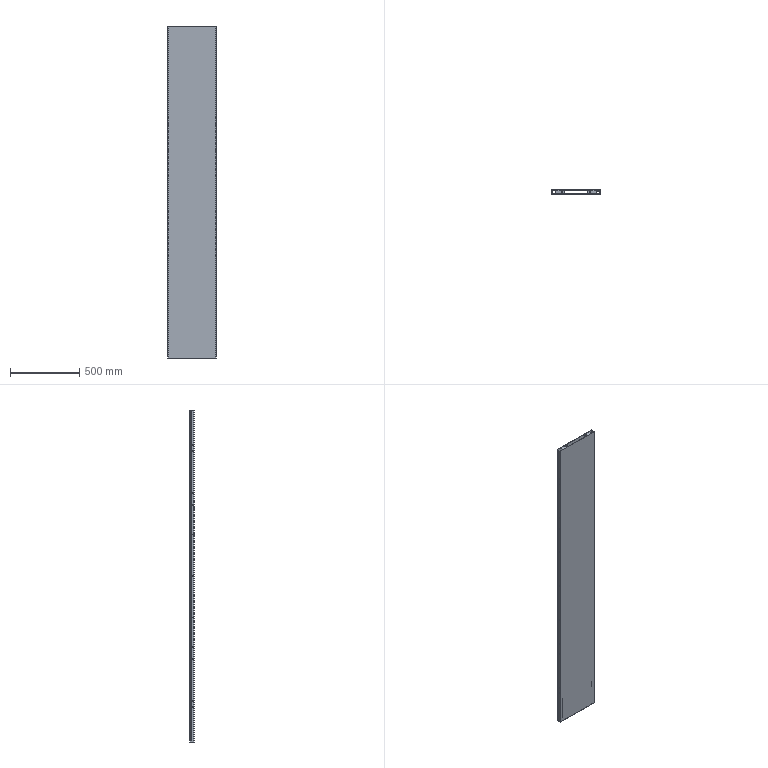Part | SolidWorks | 7 solids | 276 faces | box 350 x 30 x 2396 mm | volume 3626066 mm3 | plane 172 | cylinder 104 | commonest cylinder face diameters 6.2 x44 30 x14 0.4 x13 5 x12 4.4 x9 7 x8